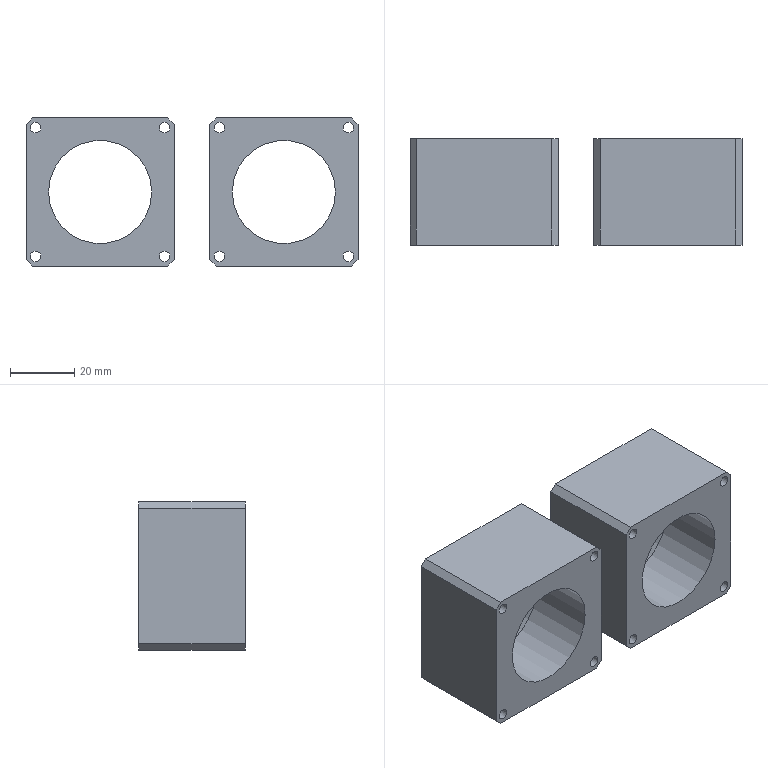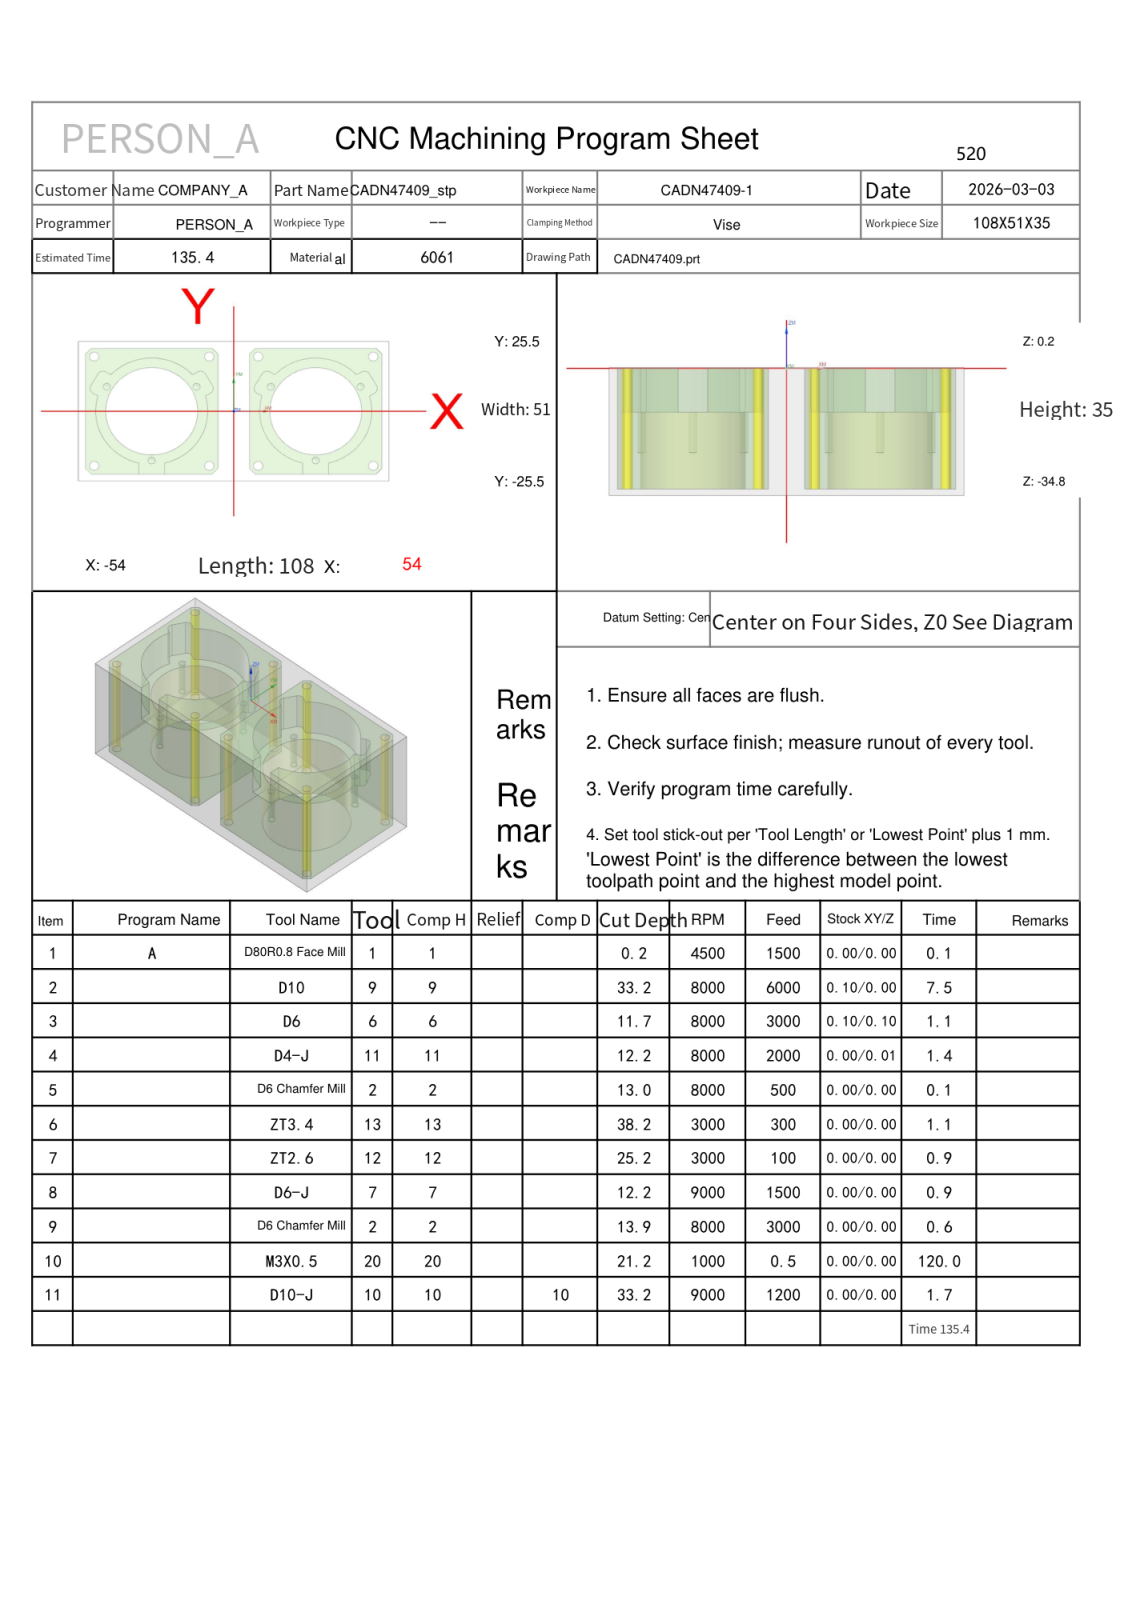NC program | NX | posted by the shop | part box 103 x 33 x 46 mm
Lines 37 to 820 of 11287:
N2 T09 M06
(D10  D=10. R=0. H=09 ce=0.10 di=0.00)
G00 G90 G54 X28.5 Y28.1 M03 S8000
G43 H09 Z50.
M08
Z.5
G01 X49.5 Z.421 F6000.
G02 X53.106 Y26.606 Z.406 I0.0 J-5.1
G01 X55.106 Y24.606 Z.395
G02 X56.6 Y21. Z.38 I-3.606 J-3.606
G01 Y-21. Z.221
G02 X55.106 Y-24.606 Z.206 I-5.1 J0.0
G01 X53.106 Y-26.606 Z.196
G02 X49.5 Y-28.1 Z.18 I-3.606 J3.606
G01 X7.5 Z.022
G02 X3.894 Y-26.606 Z.007 I0.0 J5.1
G01 X1.894 Y-24.606 Z-.004
G02 X.4 Y-21. Z-.019 I3.606 J3.606
G01 Y21. Z-.177
G02 X1.894 Y24.606 Z-.193 I5.1 J0.0
G01 X3.894 Y26.606 Z-.203
G02 X7.5 Y28.1 Z-.218 I3.606 J-3.606
G01 X49.5 Z-.377
G02 X53.106 Y26.606 Z-.392 I0.0 J-5.1
G01 X55.106 Y24.606 Z-.403
G02 X56.6 Y21. Z-.418 I-3.606 J-3.606
G01 Y-21. Z-.576
G02 X55.106 Y-24.606 Z-.591 I-5.1 J0.0
G01 X53.106 Y-26.606 Z-.602
G02 X49.5 Y-28.1 Z-.617 I-3.606 J3.606
G01 X7.5 Z-.776
G02 X3.894 Y-26.606 Z-.791 I0.0 J5.1
G01 X1.894 Y-24.606 Z-.801
G02 X.4 Y-21. Z-.817 I3.606 J3.606
G01 Y21. Z-.975
G02 X1.894 Y24.606 Z-.99 I5.1 J0.0
G01 X3.894 Y26.606 Z-1.001
G02 X7.5 Y28.1 Z-1.016 I3.606 J-3.606
G01 X49.5 Z-1.174
G02 X53.106 Y26.606 Z-1.19 I0.0 J-5.1
G01 X55.106 Y24.606 Z-1.2
G02 X56.6 Y21. Z-1.215 I-3.606 J-3.606
G01 Y-21. Z-1.374
G02 X55.106 Y-24.606 Z-1.389 I-5.1 J0.0
G01 X53.106 Y-26.606 Z-1.4
G02 X49.5 Y-28.1 Z-1.415 I-3.606 J3.606
G01 X7.5 Z-1.573
G02 X3.894 Y-26.606 Z-1.588 I0.0 J5.1
G01 X1.894 Y-24.606 Z-1.599
G02 X.4 Y-21. Z-1.614 I3.606 J3.606
G01 Y21. Z-1.773
G02 X1.894 Y24.606 Z-1.788 I5.1 J0.0
G01 X3.894 Y26.606 Z-1.798
G02 X7.5 Y28.1 Z-1.814 I3.606 J-3.606
G01 X49.5 Z-1.972
G02 X53.106 Y26.606 Z-1.987 I0.0 J-5.1
G01 X55.106 Y24.606 Z-1.998
G02 X56.6 Y21. Z-2.013 I-3.606 J-3.606
G01 Y-21. Z-2.172
G02 X55.106 Y-24.606 Z-2.187 I-5.1 J0.0
G01 X53.106 Y-26.606 Z-2.197
G02 X49.5 Y-28.1 Z-2.212 I-3.606 J3.606
G01 X7.5 Z-2.371
G02 X3.894 Y-26.606 Z-2.386 I0.0 J5.1
G01 X1.894 Y-24.606 Z-2.397
G02 X.4 Y-21. Z-2.412 I3.606 J3.606
G01 Y21. Z-2.57
G02 X1.894 Y24.606 Z-2.585 I5.1 J0.0
G01 X3.894 Y26.606 Z-2.596
G02 X7.5 Y28.1 Z-2.611 I3.606 J-3.606
G01 X49.5 Z-2.77
G02 X53.106 Y26.606 Z-2.785 I0.0 J-5.1
G01 X55.106 Y24.606 Z-2.796
G02 X56.6 Y21. Z-2.811 I-3.606 J-3.606
G01 Y-21. Z-2.969
G02 X55.106 Y-24.606 Z-2.984 I-5.1 J0.0
G01 X53.106 Y-26.606 Z-2.995
G02 X49.5 Y-28.1 Z-3.01 I-3.606 J3.606
G01 X7.5 Z-3.169
G02 X3.894 Y-26.606 Z-3.184 I0.0 J5.1
G01 X1.894 Y-24.606 Z-3.194
G02 X.4 Y-21. Z-3.209 I3.606 J3.606
G01 Y21. Z-3.368
G02 X1.894 Y24.606 Z-3.383 I5.1 J0.0
G01 X3.894 Y26.606 Z-3.394
G02 X7.5 Y28.1 Z-3.409 I3.606 J-3.606
G01 X49.5 Z-3.567
G02 X53.106 Y26.606 Z-3.582 I0.0 J-5.1
G01 X55.106 Y24.606 Z-3.593
G02 X56.6 Y21. Z-3.608 I-3.606 J-3.606
G01 Y-21. Z-3.767
G02 X55.106 Y-24.606 Z-3.782 I-5.1 J0.0
G01 X53.106 Y-26.606 Z-3.793
G02 X49.5 Y-28.1 Z-3.808 I-3.606 J3.606
G01 X7.5 Z-3.966
G02 X3.894 Y-26.606 Z-3.981 I0.0 J5.1
G01 X1.894 Y-24.606 Z-3.992
G02 X.4 Y-21. Z-4.007 I3.606 J3.606
G01 Y21. Z-4.166
G02 X1.894 Y24.606 Z-4.181 I5.1 J0.0
G01 X3.894 Y26.606 Z-4.191
G02 X7.5 Y28.1 Z-4.206 I3.606 J-3.606
G01 X49.5 Z-4.365
G02 X53.106 Y26.606 Z-4.38 I0.0 J-5.1
G01 X55.106 Y24.606 Z-4.391
G02 X56.6 Y21. Z-4.406 I-3.606 J-3.606
G01 Y-21. Z-4.564
G02 X55.106 Y-24.606 Z-4.579 I-5.1 J0.0
G01 X53.106 Y-26.606 Z-4.59
G02 X49.5 Y-28.1 Z-4.605 I-3.606 J3.606
G01 X7.5 Z-4.764
G02 X3.894 Y-26.606 Z-4.779 I0.0 J5.1
G01 X1.894 Y-24.606 Z-4.79
G02 X.4 Y-21. Z-4.805 I3.606 J3.606
G01 Y21. Z-4.963
G02 X1.894 Y24.606 Z-4.978 I5.1 J0.0
G01 X3.894 Y26.606 Z-4.989
G02 X7.5 Y28.1 Z-5.004 I3.606 J-3.606
G01 X49.5 Z-5.163
G02 X53.106 Y26.606 Z-5.178 I0.0 J-5.1
G01 X55.106 Y24.606 Z-5.188
G02 X56.6 Y21. Z-5.203 I-3.606 J-3.606
G01 Y-21. Z-5.362
G02 X55.106 Y-24.606 Z-5.377 I-5.1 J0.0
G01 X53.106 Y-26.606 Z-5.388
G02 X49.5 Y-28.1 Z-5.403 I-3.606 J3.606
G01 X7.5 Z-5.561
G02 X3.894 Y-26.606 Z-5.577 I0.0 J5.1
G01 X1.894 Y-24.606 Z-5.587
G02 X.4 Y-21. Z-5.602 I3.606 J3.606
G01 Y21. Z-5.761
G02 X1.894 Y24.606 Z-5.776 I5.1 J0.0
G01 X3.894 Y26.606 Z-5.787
G02 X7.5 Y28.1 Z-5.802 I3.606 J-3.606
G01 X49.5 Z-5.96
G02 X53.106 Y26.606 Z-5.975 I0.0 J-5.1
G01 X55.106 Y24.606 Z-5.986
G02 X56.6 Y21. Z-6.001 I-3.606 J-3.606
G01 Y-21. Z-6.16
G02 X55.106 Y-24.606 Z-6.175 I-5.1 J0.0
G01 X53.106 Y-26.606 Z-6.185
G02 X49.5 Y-28.1 Z-6.201 I-3.606 J3.606
G01 X7.5 Z-6.359
G02 X3.894 Y-26.606 Z-6.374 I0.0 J5.1
G01 X1.894 Y-24.606 Z-6.385
G02 X.4 Y-21. Z-6.4 I3.606 J3.606
G01 Y21. Z-6.558
G02 X1.894 Y24.606 Z-6.574 I5.1 J0.0
G01 X3.894 Y26.606 Z-6.584
G02 X7.5 Y28.1 Z-6.599 I3.606 J-3.606
G01 X49.5 Z-6.758
G02 X53.106 Y26.606 Z-6.773 I0.0 J-5.1
G01 X55.106 Y24.606 Z-6.784
G02 X56.6 Y21. Z-6.799 I-3.606 J-3.606
G01 Y-21. Z-6.957
G02 X55.106 Y-24.606 Z-6.972 I-5.1 J0.0
G01 X53.106 Y-26.606 Z-6.983
G02 X49.5 Y-28.1 Z-6.998 I-3.606 J3.606
G01 X7.5 Z-7.157
G02 X3.894 Y-26.606 Z-7.172 I0.0 J5.1
G01 X1.894 Y-24.606 Z-7.182
G02 X.4 Y-21. Z-7.198 I3.606 J3.606
G01 Y21. Z-7.356
G02 X1.894 Y24.606 Z-7.371 I5.1 J0.0
G01 X3.894 Y26.606 Z-7.382
G02 X7.5 Y28.1 Z-7.397 I3.606 J-3.606
G01 X49.5 Z-7.555
G02 X53.106 Y26.606 Z-7.571 I0.0 J-5.1
G01 X55.106 Y24.606 Z-7.581
G02 X56.6 Y21. Z-7.596 I-3.606 J-3.606
G01 Y-21. Z-7.755
G02 X55.106 Y-24.606 Z-7.77 I-5.1 J0.0
G01 X53.106 Y-26.606 Z-7.781
G02 X49.5 Y-28.1 Z-7.796 I-3.606 J3.606
G01 X7.5 Z-7.954
G02 X3.894 Y-26.606 Z-7.969 I0.0 J5.1
G01 X1.894 Y-24.606 Z-7.98
G02 X.4 Y-21. Z-7.995 I3.606 J3.606
G01 Y21. Z-8.154
G02 X1.894 Y24.606 Z-8.169 I5.1 J0.0
G01 X3.894 Y26.606 Z-8.179
G02 X7.5 Y28.1 Z-8.195 I3.606 J-3.606
G01 X49.5 Z-8.353
G02 X53.106 Y26.606 Z-8.368 I0.0 J-5.1
G01 X55.106 Y24.606 Z-8.379
G02 X56.6 Y21. Z-8.394 I-3.606 J-3.606
G01 Y-21. Z-8.552
G02 X55.106 Y-24.606 Z-8.568 I-5.1 J0.0
G01 X53.106 Y-26.606 Z-8.578
G02 X49.5 Y-28.1 Z-8.593 I-3.606 J3.606
G01 X7.5 Z-8.752
G02 X3.894 Y-26.606 Z-8.767 I0.0 J5.1
G01 X1.894 Y-24.606 Z-8.778
G02 X.4 Y-21. Z-8.793 I3.606 J3.606
G01 Y21. Z-8.951
G02 X1.894 Y24.606 Z-8.966 I5.1 J0.0
G01 X3.894 Y26.606 Z-8.977
G02 X7.5 Y28.1 Z-8.992 I3.606 J-3.606
G01 X49.5 Z-9.151
G02 X53.106 Y26.606 Z-9.166 I0.0 J-5.1
G01 X55.106 Y24.606 Z-9.176
G02 X56.6 Y21. Z-9.192 I-3.606 J-3.606
G01 Y-21. Z-9.35
G02 X55.106 Y-24.606 Z-9.365 I-5.1 J0.0
G01 X53.106 Y-26.606 Z-9.376
G02 X49.5 Y-28.1 Z-9.391 I-3.606 J3.606
G01 X7.5 Z-9.549
G02 X3.894 Y-26.606 Z-9.565 I0.0 J5.1
G01 X1.894 Y-24.606 Z-9.575
G02 X.4 Y-21. Z-9.59 I3.606 J3.606
G01 Y21. Z-9.749
G02 X1.894 Y24.606 Z-9.764 I5.1 J0.0
G01 X3.894 Y26.606 Z-9.775
G02 X7.5 Y28.1 Z-9.79 I3.606 J-3.606
G01 X49.5 Z-9.948
G02 X53.106 Y26.606 Z-9.963 I0.0 J-5.1
G01 X55.106 Y24.606 Z-9.974
G02 X56.6 Y21. Z-9.989 I-3.606 J-3.606
G01 Y-21. Z-10.148
G02 X55.106 Y-24.606 Z-10.163 I-5.1 J0.0
G01 X53.106 Y-26.606 Z-10.173
G02 X49.5 Y-28.1 Z-10.189 I-3.606 J3.606
G01 X7.5 Z-10.347
G02 X3.894 Y-26.606 Z-10.362 I0.0 J5.1
G01 X1.894 Y-24.606 Z-10.373
G02 X.4 Y-21. Z-10.388 I3.606 J3.606
G01 Y21. Z-10.547
G02 X1.894 Y24.606 Z-10.562 I5.1 J0.0
G01 X3.894 Y26.606 Z-10.572
G02 X7.5 Y28.1 Z-10.587 I3.606 J-3.606
G01 X49.5 Z-10.746
G02 X53.106 Y26.606 Z-10.761 I0.0 J-5.1
G01 X55.106 Y24.606 Z-10.772
G02 X56.6 Y21. Z-10.787 I-3.606 J-3.606
G01 Y-21. Z-10.945
G02 X55.106 Y-24.606 Z-10.96 I-5.1 J0.0
G01 X53.106 Y-26.606 Z-10.971
G02 X49.5 Y-28.1 Z-10.986 I-3.606 J3.606
G01 X7.5 Z-11.145
G02 X3.894 Y-26.606 Z-11.16 I0.0 J5.1
G01 X1.894 Y-24.606 Z-11.171
G02 X.4 Y-21. Z-11.186 I3.606 J3.606
G01 Y21. Z-11.344
G02 X1.894 Y24.606 Z-11.359 I5.1 J0.0
G01 X3.894 Y26.606 Z-11.37
G02 X7.5 Y28.1 Z-11.385 I3.606 J-3.606
G01 X49.5 Z-11.544
G02 X53.106 Y26.606 Z-11.559 I0.0 J-5.1
G01 X55.106 Y24.606 Z-11.569
G02 X56.6 Y21. Z-11.584 I-3.606 J-3.606
G01 Y-21. Z-11.743
G02 X55.106 Y-24.606 Z-11.758 I-5.1 J0.0
G01 X53.106 Y-26.606 Z-11.769
G02 X49.5 Y-28.1 Z-11.784 I-3.606 J3.606
G01 X7.5 Z-11.942
G02 X3.894 Y-26.606 Z-11.957 I0.0 J5.1
G01 X1.894 Y-24.606 Z-11.968
G02 X.4 Y-21. Z-11.983 I3.606 J3.606
G01 Y21. Z-12.142
G02 X1.894 Y24.606 Z-12.157 I5.1 J0.0
G01 X3.894 Y26.606 Z-12.168
G02 X7.5 Y28.1 Z-12.183 I3.606 J-3.606
G01 X49.5 Z-12.341
G02 X53.106 Y26.606 Z-12.356 I0.0 J-5.1
G01 X55.106 Y24.606 Z-12.367
G02 X56.6 Y21. Z-12.382 I-3.606 J-3.606
G01 Y-21. Z-12.541
G02 X55.106 Y-24.606 Z-12.556 I-5.1 J0.0
G01 X53.106 Y-26.606 Z-12.566
G02 X49.5 Y-28.1 Z-12.581 I-3.606 J3.606
G01 X7.5 Z-12.74
G02 X3.894 Y-26.606 Z-12.755 I0.0 J5.1
G01 X1.894 Y-24.606 Z-12.766
G02 X.4 Y-21. Z-12.781 I3.606 J3.606
G01 Y21. Z-12.939
G02 X1.894 Y24.606 Z-12.954 I5.1 J0.0
G01 X3.894 Y26.606 Z-12.965
G02 X7.5 Y28.1 Z-12.98 I3.606 J-3.606
G01 X49.5 Z-13.139
G02 X53.106 Y26.606 Z-13.154 I0.0 J-5.1
G01 X55.106 Y24.606 Z-13.165
G02 X56.6 Y21. Z-13.18 I-3.606 J-3.606
G01 Y-21. Z-13.338
G02 X55.106 Y-24.606 Z-13.353 I-5.1 J0.0
G01 X53.106 Y-26.606 Z-13.364
G02 X49.5 Y-28.1 Z-13.379 I-3.606 J3.606
G01 X7.5 Z-13.538
G02 X3.894 Y-26.606 Z-13.553 I0.0 J5.1
G01 X1.894 Y-24.606 Z-13.563
G02 X.4 Y-21. Z-13.578 I3.606 J3.606
G01 Y21. Z-13.737
G02 X1.894 Y24.606 Z-13.752 I5.1 J0.0
G01 X3.894 Y26.606 Z-13.763
G02 X7.5 Y28.1 Z-13.778 I3.606 J-3.606
G01 X49.5 Z-13.936
G02 X53.106 Y26.606 Z-13.952 I0.0 J-5.1
G01 X55.106 Y24.606 Z-13.962
G02 X56.6 Y21. Z-13.977 I-3.606 J-3.606
G01 Y-21. Z-14.136
G02 X55.106 Y-24.606 Z-14.151 I-5.1 J0.0
G01 X53.106 Y-26.606 Z-14.162
G02 X49.5 Y-28.1 Z-14.177 I-3.606 J3.606
G01 X7.5 Z-14.335
G02 X3.894 Y-26.606 Z-14.35 I0.0 J5.1
G01 X1.894 Y-24.606 Z-14.361
G02 X.4 Y-21. Z-14.376 I3.606 J3.606
G01 Y21. Z-14.535
G02 X1.894 Y24.606 Z-14.55 I5.1 J0.0
G01 X3.894 Y26.606 Z-14.56
G02 X7.5 Y28.1 Z-14.576 I3.606 J-3.606
G01 X49.5 Z-14.734
G02 X53.106 Y26.606 Z-14.749 I0.0 J-5.1
G01 X55.106 Y24.606 Z-14.76
G02 X56.6 Y21. Z-14.775 I-3.606 J-3.606
G01 Y-21. Z-14.933
G02 X55.106 Y-24.606 Z-14.949 I-5.1 J0.0
G01 X53.106 Y-26.606 Z-14.959
G02 X49.5 Y-28.1 Z-14.974 I-3.606 J3.606
G01 X7.5 Z-15.133
G02 X3.894 Y-26.606 Z-15.148 I0.0 J5.1
G01 X1.894 Y-24.606 Z-15.159
G02 X.4 Y-21. Z-15.174 I3.606 J3.606
G01 Y21. Z-15.332
G02 X1.894 Y24.606 Z-15.347 I5.1 J0.0
G01 X3.894 Y26.606 Z-15.358
G02 X7.5 Y28.1 Z-15.373 I3.606 J-3.606
G01 X49.5 Z-15.532
G02 X53.106 Y26.606 Z-15.547 I0.0 J-5.1
G01 X55.106 Y24.606 Z-15.557
G02 X56.6 Y21. Z-15.573 I-3.606 J-3.606
G01 Y-21. Z-15.731
G02 X55.106 Y-24.606 Z-15.746 I-5.1 J0.0
G01 X53.106 Y-26.606 Z-15.757
G02 X49.5 Y-28.1 Z-15.772 I-3.606 J3.606
G01 X7.5 Z-15.93
G02 X3.894 Y-26.606 Z-15.946 I0.0 J5.1
G01 X1.894 Y-24.606 Z-15.956
G02 X.4 Y-21. Z-15.971 I3.606 J3.606
G01 Y21. Z-16.13
G02 X1.894 Y24.606 Z-16.145 I5.1 J0.0
G01 X3.894 Y26.606 Z-16.156
G02 X7.5 Y28.1 Z-16.171 I3.606 J-3.606
G01 X49.5 Z-16.329
G02 X53.106 Y26.606 Z-16.344 I0.0 J-5.1
G01 X55.106 Y24.606 Z-16.355
G02 X56.6 Y21. Z-16.37 I-3.606 J-3.606
G01 Y-21. Z-16.529
G02 X55.106 Y-24.606 Z-16.544 I-5.1 J0.0
G01 X53.106 Y-26.606 Z-16.554
G02 X49.5 Y-28.1 Z-16.57 I-3.606 J3.606
G01 X7.5 Z-16.728
G02 X3.894 Y-26.606 Z-16.743 I0.0 J5.1
G01 X1.894 Y-24.606 Z-16.754
G02 X.4 Y-21. Z-16.769 I3.606 J3.606
G01 Y21. Z-16.927
G02 X1.894 Y24.606 Z-16.943 I5.1 J0.0
G01 X3.894 Y26.606 Z-16.953
G02 X7.5 Y28.1 Z-16.968 I3.606 J-3.606
G01 X49.5 Z-17.127
G02 X53.106 Y26.606 Z-17.142 I0.0 J-5.1
G01 X55.106 Y24.606 Z-17.153
G02 X56.6 Y21. Z-17.168 I-3.606 J-3.606
G01 Y-21. Z-17.326
G02 X55.106 Y-24.606 Z-17.341 I-5.1 J0.0
G01 X53.106 Y-26.606 Z-17.352
G02 X49.5 Y-28.1 Z-17.367 I-3.606 J3.606
G01 X7.5 Z-17.526
G02 X3.894 Y-26.606 Z-17.541 I0.0 J5.1
G01 X1.894 Y-24.606 Z-17.551
G02 X.4 Y-21. Z-17.567 I3.606 J3.606
G01 Y21. Z-17.725
G02 X1.894 Y24.606 Z-17.74 I5.1 J0.0
G01 X3.894 Y26.606 Z-17.751
G02 X7.5 Y28.1 Z-17.766 I3.606 J-3.606
G01 X49.5 Z-17.924
G02 X53.106 Y26.606 Z-17.94 I0.0 J-5.1
G01 X55.106 Y24.606 Z-17.95
G02 X56.6 Y21. Z-17.965 I-3.606 J-3.606
G01 Y-21. Z-18.124
G02 X55.106 Y-24.606 Z-18.139 I-5.1 J0.0
G01 X53.106 Y-26.606 Z-18.15
G02 X49.5 Y-28.1 Z-18.165 I-3.606 J3.606
G01 X7.5 Z-18.323
G02 X3.894 Y-26.606 Z-18.338 I0.0 J5.1
G01 X1.894 Y-24.606 Z-18.349
G02 X.4 Y-21. Z-18.364 I3.606 J3.606
G01 Y21. Z-18.523
G02 X1.894 Y24.606 Z-18.538 I5.1 J0.0
G01 X3.894 Y26.606 Z-18.548
G02 X7.5 Y28.1 Z-18.564 I3.606 J-3.606
G01 X49.5 Z-18.722
G02 X53.106 Y26.606 Z-18.737 I0.0 J-5.1
G01 X55.106 Y24.606 Z-18.748
G02 X56.6 Y21. Z-18.763 I-3.606 J-3.606
G01 Y-21. Z-18.922
G02 X55.106 Y-24.606 Z-18.937 I-5.1 J0.0
G01 X53.106 Y-26.606 Z-18.947
G02 X49.5 Y-28.1 Z-18.962 I-3.606 J3.606
G01 X7.5 Z-19.121
G02 X3.894 Y-26.606 Z-19.136 I0.0 J5.1
G01 X1.894 Y-24.606 Z-19.147
G02 X.4 Y-21. Z-19.162 I3.606 J3.606
G01 Y21. Z-19.32
G02 X1.894 Y24.606 Z-19.335 I5.1 J0.0
G01 X3.894 Y26.606 Z-19.346
G02 X7.5 Y28.1 Z-19.361 I3.606 J-3.606
G01 X49.5 Z-19.52
G02 X53.106 Y26.606 Z-19.535 I0.0 J-5.1
G01 X55.106 Y24.606 Z-19.546
G02 X56.6 Y21. Z-19.561 I-3.606 J-3.606
G01 Y-21. Z-19.719
G02 X55.106 Y-24.606 Z-19.734 I-5.1 J0.0
G01 X53.106 Y-26.606 Z-19.745
G02 X49.5 Y-28.1 Z-19.76 I-3.606 J3.606
G01 X7.5 Z-19.919
G02 X3.894 Y-26.606 Z-19.934 I0.0 J5.1
G01 X1.894 Y-24.606 Z-19.944
G02 X.4 Y-21. Z-19.959 I3.606 J3.606
G01 Y21. Z-20.118
G02 X1.894 Y24.606 Z-20.133 I5.1 J0.0
G01 X3.894 Y26.606 Z-20.144
G02 X7.5 Y28.1 Z-20.159 I3.606 J-3.606
G01 X49.5 Z-20.317
G02 X53.106 Y26.606 Z-20.332 I0.0 J-5.1
G01 X55.106 Y24.606 Z-20.343
G02 X56.6 Y21. Z-20.358 I-3.606 J-3.606
G01 Y-21. Z-20.517
G02 X55.106 Y-24.606 Z-20.532 I-5.1 J0.0
G01 X53.106 Y-26.606 Z-20.543
G02 X49.5 Y-28.1 Z-20.558 I-3.606 J3.606
G01 X7.5 Z-20.716
G02 X3.894 Y-26.606 Z-20.731 I0.0 J5.1
G01 X1.894 Y-24.606 Z-20.742
G02 X.4 Y-21. Z-20.757 I3.606 J3.606
G01 Y21. Z-20.916
G02 X1.894 Y24.606 Z-20.931 I5.1 J0.0
G01 X3.894 Y26.606 Z-20.941
G02 X7.5 Y28.1 Z-20.956 I3.606 J-3.606
G01 X49.5 Z-21.115
G02 X53.106 Y26.606 Z-21.13 I0.0 J-5.1
G01 X55.106 Y24.606 Z-21.141
G02 X56.6 Y21. Z-21.156 I-3.606 J-3.606
G01 Y-21. Z-21.314
G02 X55.106 Y-24.606 Z-21.329 I-5.1 J0.0
G01 X53.106 Y-26.606 Z-21.34
G02 X49.5 Y-28.1 Z-21.355 I-3.606 J3.606
G01 X7.5 Z-21.514
G02 X3.894 Y-26.606 Z-21.529 I0.0 J5.1
G01 X1.894 Y-24.606 Z-21.54
G02 X.4 Y-21. Z-21.555 I3.606 J3.606
G01 Y21. Z-21.713
G02 X1.894 Y24.606 Z-21.728 I5.1 J0.0
G01 X3.894 Y26.606 Z-21.739
G02 X7.5 Y28.1 Z-21.754 I3.606 J-3.606
G01 X49.5 Z-21.913
G02 X53.106 Y26.606 Z-21.928 I0.0 J-5.1
G01 X55.106 Y24.606 Z-21.938
G02 X56.6 Y21. Z-21.953 I-3.606 J-3.606
G01 Y-21. Z-22.112
G02 X55.106 Y-24.606 Z-22.127 I-5.1 J0.0
G01 X53.106 Y-26.606 Z-22.138
G02 X49.5 Y-28.1 Z-22.153 I-3.606 J3.606
G01 X7.5 Z-22.311
G02 X3.894 Y-26.606 Z-22.327 I0.0 J5.1
G01 X1.894 Y-24.606 Z-22.337
G02 X.4 Y-21. Z-22.352 I3.606 J3.606
G01 Y21. Z-22.511
G02 X1.894 Y24.606 Z-22.526 I5.1 J0.0
G01 X3.894 Y26.606 Z-22.537
G02 X7.5 Y28.1 Z-22.552 I3.606 J-3.606
G01 X49.5 Z-22.71
G02 X53.106 Y26.606 Z-22.725 I0.0 J-5.1
G01 X55.106 Y24.606 Z-22.736
G02 X56.6 Y21. Z-22.751 I-3.606 J-3.606
G01 Y-21. Z-22.91
G02 X55.106 Y-24.606 Z-22.925 I-5.1 J0.0
G01 X53.106 Y-26.606 Z-22.935
G02 X49.5 Y-28.1 Z-22.951 I-3.606 J3.606
G01 X7.5 Z-23.109
G02 X3.894 Y-26.606 Z-23.124 I0.0 J5.1
G01 X1.894 Y-24.606 Z-23.135
G02 X.4 Y-21. Z-23.15 I3.606 J3.606
G01 Y21. Z-23.308
G02 X1.894 Y24.606 Z-23.324 I5.1 J0.0
G01 X3.894 Y26.606 Z-23.334
G02 X7.5 Y28.1 Z-23.349 I3.606 J-3.606
G01 X49.5 Z-23.508
G02 X53.106 Y26.606 Z-23.523 I0.0 J-5.1
G01 X55.106 Y24.606 Z-23.534
G02 X56.6 Y21. Z-23.549 I-3.606 J-3.606
G01 Y-21. Z-23.707
G02 X55.106 Y-24.606 Z-23.722 I-5.1 J0.0
G01 X53.106 Y-26.606 Z-23.733
G02 X49.5 Y-28.1 Z-23.748 I-3.606 J3.606
G01 X7.5 Z-23.907
G02 X3.894 Y-26.606 Z-23.922 I0.0 J5.1
G01 X1.894 Y-24.606 Z-23.932
G02 X.4 Y-21. Z-23.948 I3.606 J3.606
G01 Y21. Z-24.106
G02 X1.894 Y24.606 Z-24.121 I5.1 J0.0
G01 X3.894 Y26.606 Z-24.132
G02 X7.5 Y28.1 Z-24.147 I3.606 J-3.606
G01 X49.5 Z-24.305
G02 X53.106 Y26.606 Z-24.321 I0.0 J-5.1
G01 X55.106 Y24.606 Z-24.331
G02 X56.6 Y21. Z-24.346 I-3.606 J-3.606
G01 Y-21. Z-24.505
G02 X55.106 Y-24.606 Z-24.52 I-5.1 J0.0
G01 X53.106 Y-26.606 Z-24.531
G02 X49.5 Y-28.1 Z-24.546 I-3.606 J3.606
G01 X7.5 Z-24.704
G02 X3.894 Y-26.606 Z-24.719 I0.0 J5.1
G01 X1.894 Y-24.606 Z-24.73
G02 X.4 Y-21. Z-24.745 I3.606 J3.606
G01 Y21. Z-24.904
G02 X1.894 Y24.606 Z-24.919 I5.1 J0.0
G01 X3.894 Y26.606 Z-24.929
G02 X7.5 Y28.1 Z-24.945 I3.606 J-3.606
G01 X49.5 Z-25.103
G02 X53.106 Y26.606 Z-25.118 I0.0 J-5.1
G01 X55.106 Y24.606 Z-25.129
G02 X56.6 Y21. Z-25.144 I-3.606 J-3.606
G01 Y-21. Z-25.302
G02 X55.106 Y-24.606 Z-25.318 I-5.1 J0.0
G01 X53.106 Y-26.606 Z-25.328
G02 X49.5 Y-28.1 Z-25.343 I-3.606 J3.606
G01 X7.5 Z-25.502
G02 X3.894 Y-26.606 Z-25.517 I0.0 J5.1
G01 X1.894 Y-24.606 Z-25.528
G02 X.4 Y-21. Z-25.543 I3.606 J3.606
G01 Y21. Z-25.701
G02 X1.894 Y24.606 Z-25.716 I5.1 J0.0
G01 X3.894 Y26.606 Z-25.727
G02 X7.5 Y28.1 Z-25.742 I3.606 J-3.606
G01 X49.5 Z-25.901
G02 X53.106 Y26.606 Z-25.916 I0.0 J-5.1
G01 X55.106 Y24.606 Z-25.926
G02 X56.6 Y21. Z-25.942 I-3.606 J-3.606
G01 Y-21. Z-26.1
G02 X55.106 Y-24.606 Z-26.115 I-5.1 J0.0
G01 X53.106 Y-26.606 Z-26.126
G02 X49.5 Y-28.1 Z-26.141 I-3.606 J3.606
G01 X7.5 Z-26.299
G02 X3.894 Y-26.606 Z-26.315 I0.0 J5.1
G01 X1.894 Y-24.606 Z-26.325
G02 X.4 Y-21. Z-26.34 I3.606 J3.606
G01 Y21. Z-26.499
G02 X1.894 Y24.606 Z-26.514 I5.1 J0.0
G01 X3.894 Y26.606 Z-26.525
G02 X7.5 Y28.1 Z-26.54 I3.606 J-3.606
G01 X49.5 Z-26.698
G02 X53.106 Y26.606 Z-26.713 I0.0 J-5.1
G01 X55.106 Y24.606 Z-26.724
G02 X56.6 Y21. Z-26.739 I-3.606 J-3.606
G01 Y-21. Z-26.898
G02 X55.106 Y-24.606 Z-26.913 I-5.1 J0.0
G01 X53.106 Y-26.606 Z-26.923
G02 X49.5 Y-28.1 Z-26.939 I-3.606 J3.606
G01 X7.5 Z-27.097
G02 X3.894 Y-26.606 Z-27.112 I0.0 J5.1
G01 X1.894 Y-24.606 Z-27.123
G02 X.4 Y-21. Z-27.138 I3.606 J3.606
G01 Y21. Z-27.297
G02 X1.894 Y24.606 Z-27.312 I5.1 J0.0
G01 X3.894 Y26.606 Z-27.322
G02 X7.5 Y28.1 Z-27.337 I3.606 J-3.606
G01 X49.5 Z-27.496
G02 X53.106 Y26.606 Z-27.511 I0.0 J-5.1
G01 X55.106 Y24.606 Z-27.522
G02 X56.6 Y21. Z-27.537 I-3.606 J-3.606
G01 Y-21. Z-27.695
G02 X55.106 Y-24.606 Z-27.71 I-5.1 J0.0
G01 X53.106 Y-26.606 Z-27.721
G02 X49.5 Y-28.1 Z-27.736 I-3.606 J3.606
G01 X7.5 Z-27.895
G02 X3.894 Y-26.606 Z-27.91 I0.0 J5.1
G01 X1.894 Y-24.606 Z-27.921
G02 X.4 Y-21. Z-27.936 I3.606 J3.606
G01 Y21. Z-28.094
G02 X1.894 Y24.606 Z-28.109 I5.1 J0.0
G01 X3.894 Y26.606 Z-28.12
G02 X7.5 Y28.1 Z-28.135 I3.606 J-3.606
G01 X49.5 Z-28.294
G02 X53.106 Y26.606 Z-28.309 I0.0 J-5.1
G01 X55.106 Y24.606 Z-28.319
G02 X56.6 Y21. Z-28.334 I-3.606 J-3.606
G01 Y-21. Z-28.493
G02 X55.106 Y-24.606 Z-28.508 I-5.1 J0.0
G01 X53.106 Y-26.606 Z-28.519
G02 X49.5 Y-28.1 Z-28.534 I-3.606 J3.606
G01 X7.5 Z-28.692
G02 X3.894 Y-26.606 Z-28.707 I0.0 J5.1
G01 X1.894 Y-24.606 Z-28.718
G02 X.4 Y-21. Z-28.733 I3.606 J3.606
G01 Y21. Z-28.892
G02 X1.894 Y24.606 Z-28.907 I5.1 J0.0
G01 X3.894 Y26.606 Z-28.918
G02 X7.5 Y28.1 Z-28.933 I3.606 J-3.606
G01 X49.5 Z-29.091
G02 X53.106 Y26.606 Z-29.106 I0.0 J-5.1
G01 X55.106 Y24.606 Z-29.117
G02 X56.6 Y21. Z-29.132 I-3.606 J-3.606
G01 Y-21. Z-29.291
G02 X55.106 Y-24.606 Z-29.306 I-5.1 J0.0
G01 X53.106 Y-26.606 Z-29.316
G02 X49.5 Y-28.1 Z-29.331 I-3.606 J3.606
G01 X7.5 Z-29.49
G02 X3.894 Y-26.606 Z-29.505 I0.0 J5.1
G01 X1.894 Y-24.606 Z-29.516
G02 X.4 Y-21. Z-29.531 I3.606 J3.606
G01 Y21. Z-29.689
G02 X1.894 Y24.606 Z-29.704 I5.1 J0.0
G01 X3.894 Y26.606 Z-29.715
G02 X7.5 Y28.1 Z-29.73 I3.606 J-3.606
G01 X49.5 Z-29.889
G02 X53.106 Y26.606 Z-29.904 I0.0 J-5.1
G01 X55.106 Y24.606 Z-29.915
G02 X56.6 Y21. Z-29.93 I-3.606 J-3.606
G01 Y-21. Z-30.088
G02 X55.106 Y-24.606 Z-30.103 I-5.1 J0.0
G01 X53.106 Y-26.606 Z-30.114
G02 X49.5 Y-28.1 Z-30.129 I-3.606 J3.606
G01 X7.5 Z-30.288
G02 X3.894 Y-26.606 Z-30.303 I0.0 J5.1
G01 X1.894 Y-24.606 Z-30.313
G02 X.4 Y-21. Z-30.328 I3.606 J3.606
G01 Y21. Z-30.487
G02 X1.894 Y24.606 Z-30.502 I5.1 J0.0
G01 X3.894 Y26.606 Z-30.513
G02 X7.5 Y28.1 Z-30.528 I3.606 J-3.606
G01 X49.5 Z-30.686
G02 X53.106 Y26.606 Z-30.702 I0.0 J-5.1
G01 X55.106 Y24.606 Z-30.712
G02 X56.6 Y21. Z-30.727 I-3.606 J-3.606
G01 Y-21. Z-30.886
G02 X55.106 Y-24.606 Z-30.901 I-5.1 J0.0
G01 X53.106 Y-26.606 Z-30.912
G02 X49.5 Y-28.1 Z-30.927 I-3.606 J3.606
G01 X7.5 Z-31.085
G02 X3.894 Y-26.606 Z-31.1 I0.0 J5.1
G01 X1.894 Y-24.606 Z-31.111
G02 X.4 Y-21. Z-31.126 I3.606 J3.606
G01 Y21. Z-31.285
G02 X1.894 Y24.606 Z-31.3 I5.1 J0.0
G01 X3.894 Y26.606 Z-31.31
G02 X7.5 Y28.1 Z-31.326 I3.606 J-3.606
G01 X49.5 Z-31.484
G02 X53.106 Y26.606 Z-31.499 I0.0 J-5.1
G01 X55.106 Y24.606 Z-31.51
G02 X56.6 Y21. Z-31.525 I-3.606 J-3.606
G01 Y-21. Z-31.683
G02 X55.106 Y-24.606 Z-31.699 I-5.1 J0.0
G01 X53.106 Y-26.606 Z-31.709
G02 X49.5 Y-28.1 Z-31.724 I-3.606 J3.606
G01 X7.5 Z-31.883
G02 X3.894 Y-26.606 Z-31.898 I0.0 J5.1
G01 X1.894 Y-24.606 Z-31.909
G02 X.4 Y-21. Z-31.924 I3.606 J3.606
G01 Y21. Z-32.082
G02 X1.894 Y24.606 Z-32.097 I5.1 J0.0
G01 X3.894 Y26.606 Z-32.108
G02 X7.5 Y28.1 Z-32.123 I3.606 J-3.606
G01 X49.5 Z-32.282
G02 X53.106 Y26.606 Z-32.297 I0.0 J-5.1
G01 X55.106 Y24.606 Z-32.307
G02 X56.6 Y21. Z-32.323 I-3.606 J-3.606
G01 Y-21. Z-32.481
G02 X55.106 Y-24.606 Z-32.496 I-5.1 J0.0
G01 X53.106 Y-26.606 Z-32.507
G02 X49.5 Y-28.1 Z-32.522 I-3.606 J3.606
G01 X7.5 Z-32.68
G02 X3.894 Y-26.606 Z-32.696 I0.0 J5.1
G01 X1.894 Y-24.606 Z-32.706
G02 X.4 Y-21. Z-32.721 I3.606 J3.606
G01 Y21. Z-32.88
G02 X1.894 Y24.606 Z-32.895 I5.1 J0.0
G01 X3.894 Y26.606 Z-32.906
G02 X7.5 Y28.1 Z-32.921 I3.606 J-3.606
G01 X28.5 Z-33.
X49.5
G02 X53.106 Y26.606 I0.0 J-5.1
G01 X55.106 Y24.606
G02 X56.6 Y21. I-3.606 J-3.606
G01 Y-21.
G02 X55.106 Y-24.606 I-5.1 J0.0
G01 X53.106 Y-26.606
G02 X49.5 Y-28.1 I-3.606 J3.606
G01 X7.5
G02 X3.894 Y-26.606 I0.0 J5.1
G01 X1.894 Y-24.606
G02 X.4 Y-21. I3.606 J3.606
G01 Y21.
G02 X1.894 Y24.606 I5.1 J0.0
G01 X3.894 Y26.606
G02 X7.5 Y28.1 I3.606 J-3.606
G01 X28.5
X29.
Z-32.
G00 Z50.
X-28.5
Z.5
G01 X-7.5 Z.421
G02 X-3.894 Y26.606 Z.406 I0.0 J-5.1
G01 X-1.894 Y24.606 Z.395
G02 X-.4 Y21. Z.38 I-3.606 J-3.606
G01 Y-21. Z.221
G02 X-1.894 Y-24.606 Z.206 I-5.1 J0.0
G01 X-3.894 Y-26.606 Z.196
G02 X-7.5 Y-28.1 Z.18 I-3.606 J3.606
G01 X-49.5 Z.022
G02 X-53.106 Y-26.606 Z.007 I0.0 J5.1
G01 X-55.106 Y-24.606 Z-.004
G02 X-56.6 Y-21. Z-.019 I3.606 J3.606
G01 Y21. Z-.177
G02 X-55.106 Y24.606 Z-.193 I5.1 J0.0
G01 X-53.106 Y26.606 Z-.203
G02 X-49.5 Y28.1 Z-.218 I3.606 J-3.606
G01 X-7.5 Z-.377
G02 X-3.894 Y26.606 Z-.392 I0.0 J-5.1
G01 X-1.894 Y24.606 Z-.403
G02 X-.4 Y21. Z-.418 I-3.606 J-3.606
G01 Y-21. Z-.576
G02 X-1.894 Y-24.606 Z-.591 I-5.1 J0.0
G01 X-3.894 Y-26.606 Z-.602
G02 X-7.5 Y-28.1 Z-.617 I-3.606 J3.606
G01 X-49.5 Z-.776
G02 X-53.106 Y-26.606 Z-.791 I0.0 J5.1
G01 X-55.106 Y-24.606 Z-.801
G02 X-56.6 Y-21. Z-.817 I3.606 J3.606
G01 Y21. Z-.975
G02 X-55.106 Y24.606 Z-.99 I5.1 J0.0
G01 X-53.106 Y26.606 Z-1.001
G02 X-49.5 Y28.1 Z-1.016 I3.606 J-3.606
G01 X-7.5 Z-1.174
G02 X-3.894 Y26.606 Z-1.19 I0.0 J-5.1
G01 X-1.894 Y24.606 Z-1.2
G02 X-.4 Y21. Z-1.215 I-3.606 J-3.606
G01 Y-21. Z-1.374
G02 X-1.894 Y-24.606 Z-1.389 I-5.1 J0.0
G01 X-3.894 Y-26.606 Z-1.4
G02 X-7.5 Y-28.1 Z-1.415 I-3.606 J3.606
G01 X-49.5 Z-1.573
G02 X-53.106 Y-26.606 Z-1.588 I0.0 J5.1
G01 X-55.106 Y-24.606 Z-1.599
G02 X-56.6 Y-21. Z-1.614 I3.606 J3.606
G01 Y21. Z-1.773
G02 X-55.106 Y24.606 Z-1.788 I5.1 J0.0
G01 X-53.106 Y26.606 Z-1.798
G02 X-49.5 Y28.1 Z-1.814 I3.606 J-3.606
G01 X-7.5 Z-1.972
G02 X-3.894 Y26.606 Z-1.987 I0.0 J-5.1
G01 X-1.894 Y24.606 Z-1.998
G02 X-.4 Y21. Z-2.013 I-3.606 J-3.606
G01 Y-21. Z-2.172
G02 X-1.894 Y-24.606 Z-2.187 I-5.1 J0.0
G01 X-3.894 Y-26.606 Z-2.197
G02 X-7.5 Y-28.1 Z-2.212 I-3.606 J3.606
G01 X-49.5 Z-2.371
G02 X-53.106 Y-26.606 Z-2.386 I0.0 J5.1
G01 X-55.106 Y-24.606 Z-2.397
G02 X-56.6 Y-21. Z-2.412 I3.606 J3.606
G01 Y21. Z-2.57
G02 X-55.106 Y24.606 Z-2.585 I5.1 J0.0
G01 X-53.106 Y26.606 Z-2.596
G02 X-49.5 Y28.1 Z-2.611 I3.606 J-3.606
G01 X-7.5 Z-2.77
G02 X-3.894 Y26.606 Z-2.785 I0.0 J-5.1
G01 X-1.894 Y24.606 Z-2.796
G02 X-.4 Y21. Z-2.811 I-3.606 J-3.606
G01 Y-21. Z-2.969
G02 X-1.894 Y-24.606 Z-2.984 I-5.1 J0.0
G01 X-3.894 Y-26.606 Z-2.995
G02 X-7.5 Y-28.1 Z-3.01 I-3.606 J3.606
G01 X-49.5 Z-3.169
G02 X-53.106 Y-26.606 Z-3.184 I0.0 J5.1
G01 X-55.106 Y-24.606 Z-3.194
G02 X-56.6 Y-21. Z-3.209 I3.606 J3.606
G01 Y21. Z-3.368
G02 X-55.106 Y24.606 Z-3.383 I5.1 J0.0
G01 X-53.106 Y26.606 Z-3.394
G02 X-49.5 Y28.1 Z-3.409 I3.606 J-3.606
G01 X-7.5 Z-3.567
G02 X-3.894 Y26.606 Z-3.582 I0.0 J-5.1
G01 X-1.894 Y24.606 Z-3.593